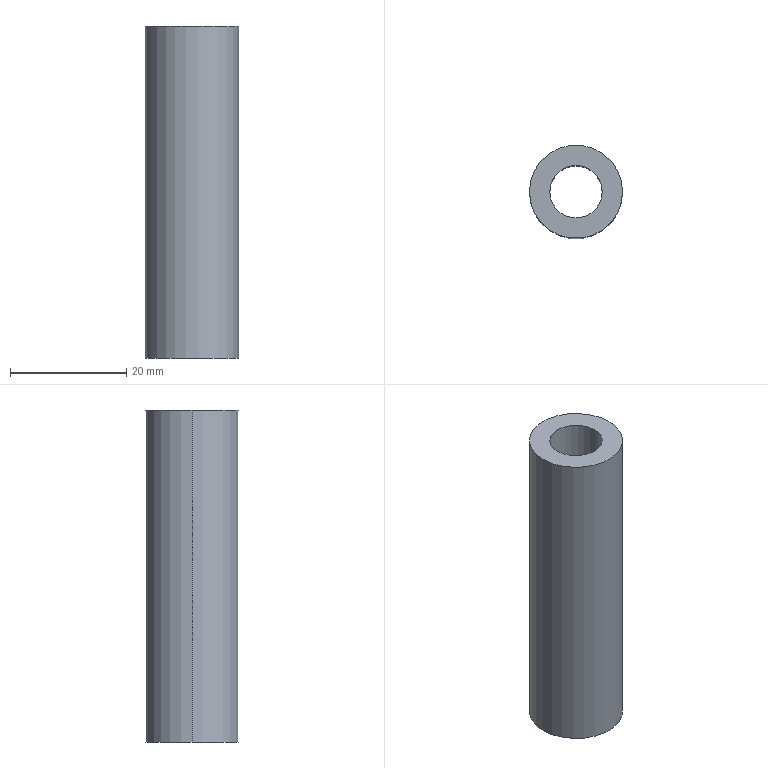Part | STEP file | PN_0014 Height locating sleeve | 1 solid | 6 faces | box 16 x 16 x 57 mm | volume 7834 mm3 | cylinder 4 | plane 2 | commonest cylinder face diameters 9 x2 16 x2
STEP:
#1=CARTESIAN_POINT('',(0.,0.,0.));
#2=DIRECTION('',(0.,0.,1.));
#3=DIRECTION('',(1.,0.,0.));
#4=AXIS2_PLACEMENT_3D('',#1,#2,#3);
#5=CARTESIAN_POINT('',(-8.,0.,57.));
#6=VERTEX_POINT('',#5);
#7=CARTESIAN_POINT('',(8.,0.,57.));
#8=VERTEX_POINT('',#7);
#9=CARTESIAN_POINT('',(0.,0.,57.));
#10=DIRECTION('',(0.,0.,-1.));
#11=DIRECTION('',(-1.,0.,0.));
#12=AXIS2_PLACEMENT_3D('',#9,#10,#11);
#13=CIRCLE('',#12,8.);
#14=CARTESIAN_POINT('',(0.,0.,57.));
#15=DIRECTION('',(0.,0.,-1.));
#16=DIRECTION('',(-1.,0.,0.));
#17=AXIS2_PLACEMENT_3D('',#14,#15,#16);
#18=CYLINDRICAL_SURFACE('',#17,8.);
#19=CARTESIAN_POINT('',(0.,0.));
#20=DIRECTION('',(1.,0.));
#21=VECTOR('',#20,1.);
#22=LINE('',#19,#21);
#23=(GEOMETRIC_REPRESENTATION_CONTEXT(2)PARAMETRIC_REPRESENTATION_CONTEXT()REPRESENTATION_CONTEXT('',''));
#24=DEFINITIONAL_REPRESENTATION('',(#22),#23);
#25=PCURVE('',#18,#24);
#26=CARTESIAN_POINT('',(0.,0.,57.));
#27=DIRECTION('',(0.,0.,1.));
#28=DIRECTION('',(1.,0.,0.));
#29=AXIS2_PLACEMENT_3D('',#26,#27,#28);
#30=PLANE('',#29);
#31=CARTESIAN_POINT('',(-8.,0.));
#32=CARTESIAN_POINT('',(-8.,13.856));
#33=CARTESIAN_POINT('',(4.,6.928));
#34=CARTESIAN_POINT('',(16.,0.));
#35=CARTESIAN_POINT('',(4.,-6.928));
#36=CARTESIAN_POINT('',(-8.,-13.856));
#37=CARTESIAN_POINT('',(-8.,0.));
#38=(BOUNDED_CURVE()B_SPLINE_CURVE(2,(#31,#32,#33,#34,#35,#36,#37),.UNSPECIFIED.,.T.,.F.)B_SPLINE_CURVE_WITH_KNOTS((1,2,2,2,2,1),(-2.094,0.,2.094,4.189,6.283,8.378),.UNSPECIFIED.)CURVE()GEOMETRIC_REPRESENTATION_ITEM()RATIONAL_B_SPLINE_CURVE((1.,0.5,1.,0.5,1.,0.5,1.))REPRESENTATION_ITEM(''));
#39=(GEOMETRIC_REPRESENTATION_CONTEXT(2)PARAMETRIC_REPRESENTATION_CONTEXT()REPRESENTATION_CONTEXT('',''));
#40=DEFINITIONAL_REPRESENTATION('',(#38),#39);
#41=PCURVE('',#30,#40);
#42=SURFACE_CURVE('',#13,(#25,#41),.PCURVE_S1.);
#43=EDGE_CURVE('',#6,#8,#42,.T.);
#44=ORIENTED_EDGE('',*,*,#43,.T.);
#45=CARTESIAN_POINT('',(8.,0.,0.));
#46=VERTEX_POINT('',#45);
#47=CARTESIAN_POINT('',(8.,0.,57.));
#48=DIRECTION('',(0.,0.,-1.));
#49=VECTOR('',#48,1.);
#50=LINE('',#47,#49);
#51=CARTESIAN_POINT('',(3.142,0.));
#52=DIRECTION('',(0.,1.));
#53=VECTOR('',#52,1.);
#54=LINE('',#51,#53);
#55=(GEOMETRIC_REPRESENTATION_CONTEXT(2)PARAMETRIC_REPRESENTATION_CONTEXT()REPRESENTATION_CONTEXT('',''));
#56=DEFINITIONAL_REPRESENTATION('',(#54),#55);
#57=PCURVE('',#18,#56);
#58=CARTESIAN_POINT('',(0.,0.,57.));
#59=DIRECTION('',(0.,0.,-1.));
#60=DIRECTION('',(-1.,0.,0.));
#61=AXIS2_PLACEMENT_3D('',#58,#59,#60);
#62=CYLINDRICAL_SURFACE('',#61,8.);
#63=CARTESIAN_POINT('',(3.142,0.));
#64=DIRECTION('',(0.,1.));
#65=VECTOR('',#64,1.);
#66=LINE('',#63,#65);
#67=(GEOMETRIC_REPRESENTATION_CONTEXT(2)PARAMETRIC_REPRESENTATION_CONTEXT()REPRESENTATION_CONTEXT('',''));
#68=DEFINITIONAL_REPRESENTATION('',(#66),#67);
#69=PCURVE('',#62,#68);
#70=SURFACE_CURVE('',#50,(#57,#69),.PCURVE_S1.);
#71=EDGE_CURVE('',#8,#46,#70,.T.);
#72=ORIENTED_EDGE('',*,*,#71,.T.);
#73=CARTESIAN_POINT('',(-8.,0.,0.));
#74=VERTEX_POINT('',#73);
#75=CARTESIAN_POINT('',(0.,0.,0.));
#76=DIRECTION('',(0.,0.,1.));
#77=DIRECTION('',(-1.,0.,0.));
#78=AXIS2_PLACEMENT_3D('',#75,#76,#77);
#79=CIRCLE('',#78,8.);
#80=CARTESIAN_POINT('',(6.283,57.));
#81=DIRECTION('',(-1.,0.));
#82=VECTOR('',#81,1.);
#83=LINE('',#80,#82);
#84=(GEOMETRIC_REPRESENTATION_CONTEXT(2)PARAMETRIC_REPRESENTATION_CONTEXT()REPRESENTATION_CONTEXT('',''));
#85=DEFINITIONAL_REPRESENTATION('',(#83),#84);
#86=PCURVE('',#18,#85);
#87=CARTESIAN_POINT('',(0.,0.,0.));
#88=DIRECTION('',(0.,0.,1.));
#89=DIRECTION('',(1.,0.,0.));
#90=AXIS2_PLACEMENT_3D('',#87,#88,#89);
#91=PLANE('',#90);
#92=CARTESIAN_POINT('',(0.,0.));
#93=DIRECTION('',(-1.,0.));
#94=AXIS2_PLACEMENT_2D('',#92,#93);
#95=CIRCLE('',#94,8.);
#96=(GEOMETRIC_REPRESENTATION_CONTEXT(2)PARAMETRIC_REPRESENTATION_CONTEXT()REPRESENTATION_CONTEXT('',''));
#97=DEFINITIONAL_REPRESENTATION('',(#95),#96);
#98=PCURVE('',#91,#97);
#99=SURFACE_CURVE('',#79,(#86,#98),.PCURVE_S1.);
#100=EDGE_CURVE('',#46,#74,#99,.T.);
#101=ORIENTED_EDGE('',*,*,#100,.T.);
#102=CARTESIAN_POINT('',(-8.,0.,57.));
#103=DIRECTION('',(0.,0.,-1.));
#104=VECTOR('',#103,1.);
#105=LINE('',#102,#104);
#106=CARTESIAN_POINT('',(0.,0.));
#107=DIRECTION('',(0.,1.));
#108=VECTOR('',#107,1.);
#109=LINE('',#106,#108);
#110=(GEOMETRIC_REPRESENTATION_CONTEXT(2)PARAMETRIC_REPRESENTATION_CONTEXT()REPRESENTATION_CONTEXT('',''));
#111=DEFINITIONAL_REPRESENTATION('',(#109),#110);
#112=PCURVE('',#18,#111);
#113=CARTESIAN_POINT('',(6.283,0.));
#114=DIRECTION('',(0.,1.));
#115=VECTOR('',#114,1.);
#116=LINE('',#113,#115);
#117=(GEOMETRIC_REPRESENTATION_CONTEXT(2)PARAMETRIC_REPRESENTATION_CONTEXT()REPRESENTATION_CONTEXT('',''));
#118=DEFINITIONAL_REPRESENTATION('',(#116),#117);
#119=PCURVE('',#62,#118);
#120=SURFACE_CURVE('',#105,(#112,#119),.PCURVE_S1.);
#121=EDGE_CURVE('',#6,#74,#120,.T.);
#122=ORIENTED_EDGE('',*,*,#121,.F.);
#123=EDGE_LOOP('',(#44,#72,#101,#122));
#124=FACE_BOUND('',#123,.T.);
#125=ADVANCED_FACE('',(#124),#18,.T.);
#126=CARTESIAN_POINT('',(-4.5,0.,57.));
#127=VERTEX_POINT('',#126);
#128=CARTESIAN_POINT('',(-4.5,0.,0.));
#129=VERTEX_POINT('',#128);
#130=CARTESIAN_POINT('',(-4.5,0.,57.));
#131=DIRECTION('',(0.,0.,-1.));
#132=VECTOR('',#131,1.);
#133=LINE('',#130,#132);
#134=CARTESIAN_POINT('',(0.,0.,57.));
#135=DIRECTION('',(0.,0.,-1.));
#136=DIRECTION('',(-1.,0.,0.));
#137=AXIS2_PLACEMENT_3D('',#134,#135,#136);
#138=CYLINDRICAL_SURFACE('',#137,4.5);
#139=CARTESIAN_POINT('',(6.283,0.));
#140=DIRECTION('',(0.,1.));
#141=VECTOR('',#140,1.);
#142=LINE('',#139,#141);
#143=(GEOMETRIC_REPRESENTATION_CONTEXT(2)PARAMETRIC_REPRESENTATION_CONTEXT()REPRESENTATION_CONTEXT('',''));
#144=DEFINITIONAL_REPRESENTATION('',(#142),#143);
#145=PCURVE('',#138,#144);
#146=CARTESIAN_POINT('',(0.,0.,57.));
#147=DIRECTION('',(0.,0.,-1.));
#148=DIRECTION('',(-1.,0.,0.));
#149=AXIS2_PLACEMENT_3D('',#146,#147,#148);
#150=CYLINDRICAL_SURFACE('',#149,4.5);
#151=CARTESIAN_POINT('',(0.,0.));
#152=DIRECTION('',(0.,1.));
#153=VECTOR('',#152,1.);
#154=LINE('',#151,#153);
#155=(GEOMETRIC_REPRESENTATION_CONTEXT(2)PARAMETRIC_REPRESENTATION_CONTEXT()REPRESENTATION_CONTEXT('',''));
#156=DEFINITIONAL_REPRESENTATION('',(#154),#155);
#157=PCURVE('',#150,#156);
#158=SURFACE_CURVE('',#133,(#145,#157),.PCURVE_S1.);
#159=EDGE_CURVE('',#127,#129,#158,.T.);
#160=ORIENTED_EDGE('',*,*,#159,.T.);
#161=CARTESIAN_POINT('',(4.5,0.,0.));
#162=VERTEX_POINT('',#161);
#163=CARTESIAN_POINT('',(0.,0.,0.));
#164=DIRECTION('',(0.,0.,-1.));
#165=DIRECTION('',(-1.,0.,0.));
#166=AXIS2_PLACEMENT_3D('',#163,#164,#165);
#167=CIRCLE('',#166,4.5);
#168=CARTESIAN_POINT('',(0.,57.));
#169=DIRECTION('',(1.,0.));
#170=VECTOR('',#169,1.);
#171=LINE('',#168,#170);
#172=(GEOMETRIC_REPRESENTATION_CONTEXT(2)PARAMETRIC_REPRESENTATION_CONTEXT()REPRESENTATION_CONTEXT('',''));
#173=DEFINITIONAL_REPRESENTATION('',(#171),#172);
#174=PCURVE('',#138,#173);
#175=CARTESIAN_POINT('',(-4.5,0.));
#176=CARTESIAN_POINT('',(-4.5,7.794));
#177=CARTESIAN_POINT('',(2.25,3.897));
#178=CARTESIAN_POINT('',(9.,0.));
#179=CARTESIAN_POINT('',(2.25,-3.897));
#180=CARTESIAN_POINT('',(-4.5,-7.794));
#181=CARTESIAN_POINT('',(-4.5,0.));
#182=(BOUNDED_CURVE()B_SPLINE_CURVE(2,(#175,#176,#177,#178,#179,#180,#181),.UNSPECIFIED.,.T.,.F.)B_SPLINE_CURVE_WITH_KNOTS((1,2,2,2,2,1),(-2.094,0.,2.094,4.189,6.283,8.378),.UNSPECIFIED.)CURVE()GEOMETRIC_REPRESENTATION_ITEM()RATIONAL_B_SPLINE_CURVE((1.,0.5,1.,0.5,1.,0.5,1.))REPRESENTATION_ITEM(''));
#183=(GEOMETRIC_REPRESENTATION_CONTEXT(2)PARAMETRIC_REPRESENTATION_CONTEXT()REPRESENTATION_CONTEXT('',''));
#184=DEFINITIONAL_REPRESENTATION('',(#182),#183);
#185=PCURVE('',#91,#184);
#186=SURFACE_CURVE('',#167,(#174,#185),.PCURVE_S1.);
#187=EDGE_CURVE('',#162,#129,#186,.T.);
#188=ORIENTED_EDGE('',*,*,#187,.F.);
#189=CARTESIAN_POINT('',(4.5,0.,57.));
#190=VERTEX_POINT('',#189);
#191=CARTESIAN_POINT('',(4.5,0.,57.));
#192=DIRECTION('',(0.,0.,-1.));
#193=VECTOR('',#192,1.);
#194=LINE('',#191,#193);
#195=CARTESIAN_POINT('',(3.142,0.));
#196=DIRECTION('',(0.,1.));
#197=VECTOR('',#196,1.);
#198=LINE('',#195,#197);
#199=(GEOMETRIC_REPRESENTATION_CONTEXT(2)PARAMETRIC_REPRESENTATION_CONTEXT()REPRESENTATION_CONTEXT('',''));
#200=DEFINITIONAL_REPRESENTATION('',(#198),#199);
#201=PCURVE('',#138,#200);
#202=CARTESIAN_POINT('',(3.142,0.));
#203=DIRECTION('',(0.,1.));
#204=VECTOR('',#203,1.);
#205=LINE('',#202,#204);
#206=(GEOMETRIC_REPRESENTATION_CONTEXT(2)PARAMETRIC_REPRESENTATION_CONTEXT()REPRESENTATION_CONTEXT('',''));
#207=DEFINITIONAL_REPRESENTATION('',(#205),#206);
#208=PCURVE('',#150,#207);
#209=SURFACE_CURVE('',#194,(#201,#208),.PCURVE_S1.);
#210=EDGE_CURVE('',#190,#162,#209,.T.);
#211=ORIENTED_EDGE('',*,*,#210,.F.);
#212=CARTESIAN_POINT('',(0.,0.,57.));
#213=DIRECTION('',(0.,0.,-1.));
#214=DIRECTION('',(-1.,0.,0.));
#215=AXIS2_PLACEMENT_3D('',#212,#213,#214);
#216=CIRCLE('',#215,4.5);
#217=CARTESIAN_POINT('',(0.,0.));
#218=DIRECTION('',(1.,0.));
#219=VECTOR('',#218,1.);
#220=LINE('',#217,#219);
#221=(GEOMETRIC_REPRESENTATION_CONTEXT(2)PARAMETRIC_REPRESENTATION_CONTEXT()REPRESENTATION_CONTEXT('',''));
#222=DEFINITIONAL_REPRESENTATION('',(#220),#221);
#223=PCURVE('',#138,#222);
#224=CARTESIAN_POINT('',(-4.5,0.));
#225=CARTESIAN_POINT('',(-4.5,7.794));
#226=CARTESIAN_POINT('',(2.25,3.897));
#227=CARTESIAN_POINT('',(9.,0.));
#228=CARTESIAN_POINT('',(2.25,-3.897));
#229=CARTESIAN_POINT('',(-4.5,-7.794));
#230=CARTESIAN_POINT('',(-4.5,0.));
#231=(BOUNDED_CURVE()B_SPLINE_CURVE(2,(#224,#225,#226,#227,#228,#229,#230),.UNSPECIFIED.,.T.,.F.)B_SPLINE_CURVE_WITH_KNOTS((1,2,2,2,2,1),(-2.094,0.,2.094,4.189,6.283,8.378),.UNSPECIFIED.)CURVE()GEOMETRIC_REPRESENTATION_ITEM()RATIONAL_B_SPLINE_CURVE((1.,0.5,1.,0.5,1.,0.5,1.))REPRESENTATION_ITEM(''));
#232=(GEOMETRIC_REPRESENTATION_CONTEXT(2)PARAMETRIC_REPRESENTATION_CONTEXT()REPRESENTATION_CONTEXT('',''));
#233=DEFINITIONAL_REPRESENTATION('',(#231),#232);
#234=PCURVE('',#30,#233);
#235=SURFACE_CURVE('',#216,(#223,#234),.PCURVE_S1.);
#236=EDGE_CURVE('',#190,#127,#235,.T.);
#237=ORIENTED_EDGE('',*,*,#236,.T.);
#238=EDGE_LOOP('',(#160,#188,#211,#237));
#239=FACE_BOUND('',#238,.F.);
#240=ADVANCED_FACE('',(#239),#138,.F.);
#241=ORIENTED_EDGE('',*,*,#71,.F.);
#242=CARTESIAN_POINT('',(0.,0.,57.));
#243=DIRECTION('',(0.,0.,-1.));
#244=DIRECTION('',(-1.,0.,0.));
#245=AXIS2_PLACEMENT_3D('',#242,#243,#244);
#246=CIRCLE('',#245,8.);
#247=CARTESIAN_POINT('',(0.,0.));
#248=DIRECTION('',(1.,0.));
#249=VECTOR('',#248,1.);
#250=LINE('',#247,#249);
#251=(GEOMETRIC_REPRESENTATION_CONTEXT(2)PARAMETRIC_REPRESENTATION_CONTEXT()REPRESENTATION_CONTEXT('',''));
#252=DEFINITIONAL_REPRESENTATION('',(#250),#251);
#253=PCURVE('',#62,#252);
#254=CARTESIAN_POINT('',(-8.,0.));
#255=CARTESIAN_POINT('',(-8.,13.856));
#256=CARTESIAN_POINT('',(4.,6.928));
#257=CARTESIAN_POINT('',(16.,0.));
#258=CARTESIAN_POINT('',(4.,-6.928));
#259=CARTESIAN_POINT('',(-8.,-13.856));
#260=CARTESIAN_POINT('',(-8.,0.));
#261=(BOUNDED_CURVE()B_SPLINE_CURVE(2,(#254,#255,#256,#257,#258,#259,#260),.UNSPECIFIED.,.T.,.F.)B_SPLINE_CURVE_WITH_KNOTS((1,2,2,2,2,1),(-2.094,0.,2.094,4.189,6.283,8.378),.UNSPECIFIED.)CURVE()GEOMETRIC_REPRESENTATION_ITEM()RATIONAL_B_SPLINE_CURVE((1.,0.5,1.,0.5,1.,0.5,1.))REPRESENTATION_ITEM(''));
#262=(GEOMETRIC_REPRESENTATION_CONTEXT(2)PARAMETRIC_REPRESENTATION_CONTEXT()REPRESENTATION_CONTEXT('',''));
#263=DEFINITIONAL_REPRESENTATION('',(#261),#262);
#264=PCURVE('',#30,#263);
#265=SURFACE_CURVE('',#246,(#253,#264),.PCURVE_S1.);
#266=EDGE_CURVE('',#8,#6,#265,.T.);
#267=ORIENTED_EDGE('',*,*,#266,.T.);
#268=ORIENTED_EDGE('',*,*,#121,.T.);
#269=CARTESIAN_POINT('',(0.,0.,0.));
#270=DIRECTION('',(0.,0.,1.));
#271=DIRECTION('',(-1.,0.,0.));
#272=AXIS2_PLACEMENT_3D('',#269,#270,#271);
#273=CIRCLE('',#272,8.);
#274=CARTESIAN_POINT('',(6.283,57.));
#275=DIRECTION('',(-1.,0.));
#276=VECTOR('',#275,1.);
#277=LINE('',#274,#276);
#278=(GEOMETRIC_REPRESENTATION_CONTEXT(2)PARAMETRIC_REPRESENTATION_CONTEXT()REPRESENTATION_CONTEXT('',''));
#279=DEFINITIONAL_REPRESENTATION('',(#277),#278);
#280=PCURVE('',#62,#279);
#281=CARTESIAN_POINT('',(0.,0.));
#282=DIRECTION('',(-1.,0.));
#283=AXIS2_PLACEMENT_2D('',#281,#282);
#284=CIRCLE('',#283,8.);
#285=(GEOMETRIC_REPRESENTATION_CONTEXT(2)PARAMETRIC_REPRESENTATION_CONTEXT()REPRESENTATION_CONTEXT('',''));
#286=DEFINITIONAL_REPRESENTATION('',(#284),#285);
#287=PCURVE('',#91,#286);
#288=SURFACE_CURVE('',#273,(#280,#287),.PCURVE_S1.);
#289=EDGE_CURVE('',#74,#46,#288,.T.);
#290=ORIENTED_EDGE('',*,*,#289,.T.);
#291=EDGE_LOOP('',(#241,#267,#268,#290));
#292=FACE_BOUND('',#291,.T.);
#293=ADVANCED_FACE('',(#292),#62,.T.);
#294=CARTESIAN_POINT('',(0.,0.,0.));
#295=DIRECTION('',(0.,0.,-1.));
#296=DIRECTION('',(-1.,0.,0.));
#297=AXIS2_PLACEMENT_3D('',#294,#295,#296);
#298=CIRCLE('',#297,4.5);
#299=CARTESIAN_POINT('',(-4.5,0.));
#300=CARTESIAN_POINT('',(-4.5,7.794));
#301=CARTESIAN_POINT('',(2.25,3.897));
#302=CARTESIAN_POINT('',(9.,0.));
#303=CARTESIAN_POINT('',(2.25,-3.897));
#304=CARTESIAN_POINT('',(-4.5,-7.794));
#305=CARTESIAN_POINT('',(-4.5,0.));
#306=(BOUNDED_CURVE()B_SPLINE_CURVE(2,(#299,#300,#301,#302,#303,#304,#305),.UNSPECIFIED.,.T.,.F.)B_SPLINE_CURVE_WITH_KNOTS((1,2,2,2,2,1),(-2.094,0.,2.094,4.189,6.283,8.378),.UNSPECIFIED.)CURVE()GEOMETRIC_REPRESENTATION_ITEM()RATIONAL_B_SPLINE_CURVE((1.,0.5,1.,0.5,1.,0.5,1.))REPRESENTATION_ITEM(''));
#307=(GEOMETRIC_REPRESENTATION_CONTEXT(2)PARAMETRIC_REPRESENTATION_CONTEXT()REPRESENTATION_CONTEXT('',''));
#308=DEFINITIONAL_REPRESENTATION('',(#306),#307);
#309=PCURVE('',#91,#308);
#310=CARTESIAN_POINT('',(0.,57.));
#311=DIRECTION('',(1.,0.));
#312=VECTOR('',#311,1.);
#313=LINE('',#310,#312);
#314=(GEOMETRIC_REPRESENTATION_CONTEXT(2)PARAMETRIC_REPRESENTATION_CONTEXT()REPRESENTATION_CONTEXT('',''));
#315=DEFINITIONAL_REPRESENTATION('',(#313),#314);
#316=PCURVE('',#150,#315);
#317=SURFACE_CURVE('',#298,(#309,#316),.PCURVE_S1.);
#318=EDGE_CURVE('',#129,#162,#317,.T.);
#319=ORIENTED_EDGE('',*,*,#318,.F.);
#320=ORIENTED_EDGE('',*,*,#187,.F.);
#321=EDGE_LOOP('',(#319,#320));
#322=FACE_BOUND('',#321,.T.);
#323=ORIENTED_EDGE('',*,*,#289,.F.);
#324=ORIENTED_EDGE('',*,*,#100,.F.);
#325=EDGE_LOOP('',(#323,#324));
#326=FACE_BOUND('',#325,.T.);
#327=ADVANCED_FACE('',(#322,#326),#91,.F.);
#328=CARTESIAN_POINT('',(0.,0.,57.));
#329=DIRECTION('',(0.,0.,-1.));
#330=DIRECTION('',(-1.,0.,0.));
#331=AXIS2_PLACEMENT_3D('',#328,#329,#330);
#332=CIRCLE('',#331,4.5);
#333=CARTESIAN_POINT('',(-4.5,0.));
#334=CARTESIAN_POINT('',(-4.5,7.794));
#335=CARTESIAN_POINT('',(2.25,3.897));
#336=CARTESIAN_POINT('',(9.,0.));
#337=CARTESIAN_POINT('',(2.25,-3.897));
#338=CARTESIAN_POINT('',(-4.5,-7.794));
#339=CARTESIAN_POINT('',(-4.5,0.));
#340=(BOUNDED_CURVE()B_SPLINE_CURVE(2,(#333,#334,#335,#336,#337,#338,#339),.UNSPECIFIED.,.T.,.F.)B_SPLINE_CURVE_WITH_KNOTS((1,2,2,2,2,1),(-2.094,0.,2.094,4.189,6.283,8.378),.UNSPECIFIED.)CURVE()GEOMETRIC_REPRESENTATION_ITEM()RATIONAL_B_SPLINE_CURVE((1.,0.5,1.,0.5,1.,0.5,1.))REPRESENTATION_ITEM(''));
#341=(GEOMETRIC_REPRESENTATION_CONTEXT(2)PARAMETRIC_REPRESENTATION_CONTEXT()REPRESENTATION_CONTEXT('',''));
#342=DEFINITIONAL_REPRESENTATION('',(#340),#341);
#343=PCURVE('',#30,#342);
#344=CARTESIAN_POINT('',(0.,0.));
#345=DIRECTION('',(1.,0.));
#346=VECTOR('',#345,1.);
#347=LINE('',#344,#346);
#348=(GEOMETRIC_REPRESENTATION_CONTEXT(2)PARAMETRIC_REPRESENTATION_CONTEXT()REPRESENTATION_CONTEXT('',''));
#349=DEFINITIONAL_REPRESENTATION('',(#347),#348);
#350=PCURVE('',#150,#349);
#351=SURFACE_CURVE('',#332,(#343,#350),.PCURVE_S1.);
#352=EDGE_CURVE('',#127,#190,#351,.T.);
#353=ORIENTED_EDGE('',*,*,#352,.T.);
#354=ORIENTED_EDGE('',*,*,#236,.T.);
#355=EDGE_LOOP('',(#353,#354));
#356=FACE_BOUND('',#355,.T.);
#357=ORIENTED_EDGE('',*,*,#43,.F.);
#358=ORIENTED_EDGE('',*,*,#266,.F.);
#359=EDGE_LOOP('',(#357,#358));
#360=FACE_BOUND('',#359,.T.);
#361=ADVANCED_FACE('',(#356,#360),#30,.T.);
#362=ORIENTED_EDGE('',*,*,#318,.F.);
#363=ORIENTED_EDGE('',*,*,#159,.F.);
#364=ORIENTED_EDGE('',*,*,#352,.T.);
#365=ORIENTED_EDGE('',*,*,#210,.T.);
#366=EDGE_LOOP('',(#362,#363,#364,#365));
#367=FACE_BOUND('',#366,.F.);
#368=ADVANCED_FACE('',(#367),#150,.F.);
#369=CLOSED_SHELL('',(#125,#240,#293,#327,#361,#368));
#370=MANIFOLD_SOLID_BREP('',#369);
#371=(LENGTH_UNIT()NAMED_UNIT(*)SI_UNIT(.MILLI.,.METRE.));
#372=UNCERTAINTY_MEASURE_WITH_UNIT(LENGTH_MEASURE(0.0000001),#371,'','');
#373=(NAMED_UNIT(*)PLANE_ANGLE_UNIT()SI_UNIT($,.RADIAN.));
#374=(NAMED_UNIT(*)SI_UNIT($,.STERADIAN.)SOLID_ANGLE_UNIT());
#375=(GEOMETRIC_REPRESENTATION_CONTEXT(3)GLOBAL_UNCERTAINTY_ASSIGNED_CONTEXT((#372))GLOBAL_UNIT_ASSIGNED_CONTEXT((#371,#373,#374))REPRESENTATION_CONTEXT('',''));
#376=ADVANCED_BREP_SHAPE_REPRESENTATION('',(#4,#370),#375);